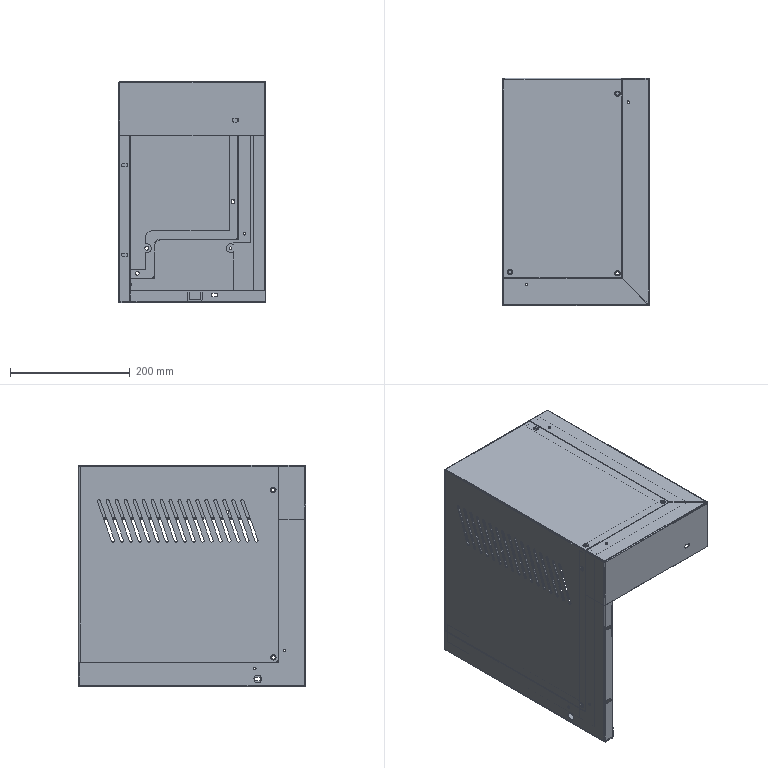Part | SolidWorks | features InContextFeatHolder 20 | 6 solids | 442 faces | box 245 x 380 x 370 mm | volume 729240 mm3 | plane 250 | cylinder 170 | cone 14 | spline 8 | commonest cylinder face diameters 5 x51 4 x39 6.4 x24 1 x15 6 x13 13 x7